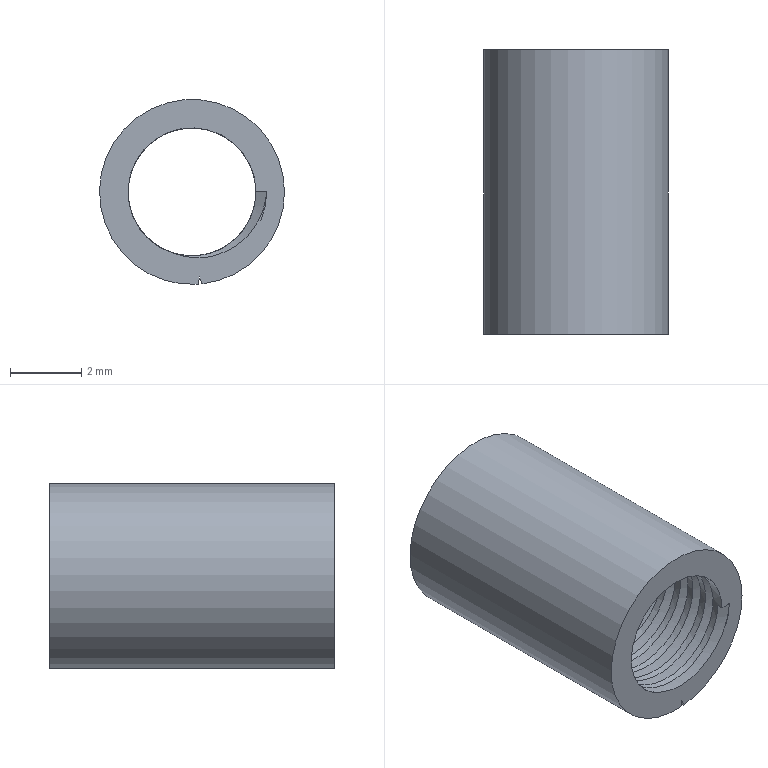Part | NX | 1 solid | 16 faces | box 5.2 x 8 x 5.2 mm | volume 80.212 mm3 | spline 8 | plane 6 | cylinder 2 | commonest cylinder face diameters 3.6 x1 5.2 x1